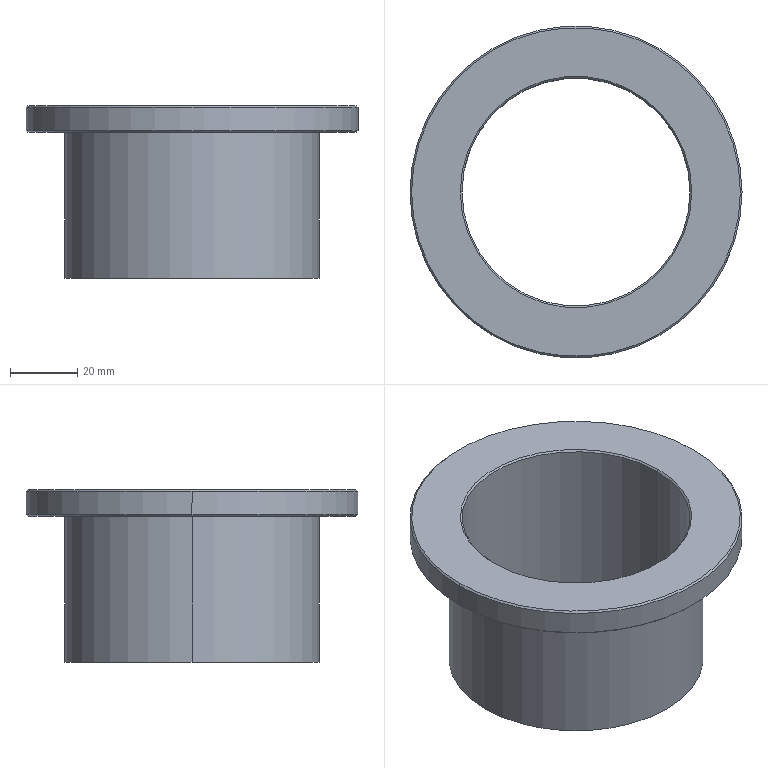Part | STEP file | 7014 Inner Spacer | 1 solid | 15 faces | box 99 x 99 x 51.5 mm | volume 71782 mm3 | cylinder 6 | cone 6 | plane 3 | commonest cylinder face diameters 68 x2 76 x2 99 x2
STEP:
#1=CARTESIAN_POINT('',(34.,0.,51.));
#2=VERTEX_POINT('',#1);
#3=CARTESIAN_POINT('',(-34.,0.,51.));
#4=VERTEX_POINT('',#3);
#5=CARTESIAN_POINT('',(0.,0.,51.));
#6=DIRECTION('',(0.,0.,-1.));
#7=DIRECTION('',(-1.,0.,0.));
#8=AXIS2_PLACEMENT_3D('',#5,#6,#7);
#9=CIRCLE('',#8,34.);
#10=EDGE_CURVE('',#2,#4,#9,.T.);
#11=ORIENTED_EDGE('',*,*,#10,.F.);
#12=CARTESIAN_POINT('',(34.,0.,0.));
#13=VERTEX_POINT('',#12);
#14=CARTESIAN_POINT('',(34.,0.,43.5));
#15=DIRECTION('',(0.,0.,-1.));
#16=VECTOR('',#15,1000.);
#17=LINE('',#14,#16);
#18=EDGE_CURVE('',#2,#13,#17,.T.);
#19=ORIENTED_EDGE('',*,*,#18,.T.);
#20=CARTESIAN_POINT('',(-34.,0.,0.));
#21=VERTEX_POINT('',#20);
#22=CARTESIAN_POINT('',(0.,0.,0.));
#23=DIRECTION('',(0.,0.,1.));
#24=DIRECTION('',(-1.,0.,0.));
#25=AXIS2_PLACEMENT_3D('',#22,#23,#24);
#26=CIRCLE('',#25,34.);
#27=EDGE_CURVE('',#21,#13,#26,.T.);
#28=ORIENTED_EDGE('',*,*,#27,.F.);
#29=CARTESIAN_POINT('',(-34.,0.,43.5));
#30=DIRECTION('',(0.,0.,-1.));
#31=VECTOR('',#30,1000.);
#32=LINE('',#29,#31);
#33=EDGE_CURVE('',#4,#21,#32,.T.);
#34=ORIENTED_EDGE('',*,*,#33,.F.);
#35=EDGE_LOOP('',(#11,#19,#28,#34));
#36=FACE_OUTER_BOUND('',#35,.T.);
#37=CARTESIAN_POINT('',(0.,0.,43.5));
#38=DIRECTION('',(0.,0.,-1.));
#39=DIRECTION('',(-1.,0.,0.));
#40=AXIS2_PLACEMENT_3D('',#37,#38,#39);
#41=CYLINDRICAL_SURFACE('',#40,34.);
#42=ADVANCED_FACE('',(#36),#41,.F.);
#43=ORIENTED_EDGE('',*,*,#10,.T.);
#44=CARTESIAN_POINT('',(-34.5,0.,51.5));
#45=VERTEX_POINT('',#44);
#46=CARTESIAN_POINT('',(-34.5,0.,51.5));
#47=DIRECTION('',(-0.7071,0.,0.7071));
#48=VECTOR('',#47,1000.);
#49=LINE('',#46,#48);
#50=EDGE_CURVE('',#4,#45,#49,.T.);
#51=ORIENTED_EDGE('',*,*,#50,.T.);
#52=CARTESIAN_POINT('',(34.5,0.,51.5));
#53=VERTEX_POINT('',#52);
#54=CARTESIAN_POINT('',(0.,0.,51.5));
#55=DIRECTION('',(0.,0.,-1.));
#56=DIRECTION('',(1.,0.,0.));
#57=AXIS2_PLACEMENT_3D('',#54,#55,#56);
#58=CIRCLE('',#57,34.5);
#59=EDGE_CURVE('',#53,#45,#58,.T.);
#60=ORIENTED_EDGE('',*,*,#59,.F.);
#61=CARTESIAN_POINT('',(34.5,0.,51.5));
#62=DIRECTION('',(0.7071,0.,0.7071));
#63=VECTOR('',#62,1000.);
#64=LINE('',#61,#63);
#65=EDGE_CURVE('',#2,#53,#64,.T.);
#66=ORIENTED_EDGE('',*,*,#65,.F.);
#67=EDGE_LOOP('',(#43,#51,#60,#66));
#68=FACE_OUTER_BOUND('',#67,.T.);
#69=CARTESIAN_POINT('',(0.,0.,51.5));
#70=DIRECTION('',(0.,0.,1.));
#71=DIRECTION('',(1.,0.,0.));
#72=AXIS2_PLACEMENT_3D('',#69,#70,#71);
#73=CONICAL_SURFACE('',#72,34.5,0.7854);
#74=ADVANCED_FACE('',(#68),#73,.F.);
#75=CARTESIAN_POINT('',(-38.,0.,43.5));
#76=VERTEX_POINT('',#75);
#77=CARTESIAN_POINT('',(38.,0.,43.5));
#78=VERTEX_POINT('',#77);
#79=CARTESIAN_POINT('',(0.,0.,43.5));
#80=DIRECTION('',(0.,0.,-1.));
#81=DIRECTION('',(-1.,0.,0.));
#82=AXIS2_PLACEMENT_3D('',#79,#80,#81);
#83=CIRCLE('',#82,38.);
#84=EDGE_CURVE('',#76,#78,#83,.T.);
#85=ORIENTED_EDGE('',*,*,#84,.T.);
#86=CARTESIAN_POINT('',(38.,0.,0.));
#87=VERTEX_POINT('',#86);
#88=CARTESIAN_POINT('',(38.,0.,43.5));
#89=DIRECTION('',(0.,0.,-1.));
#90=VECTOR('',#89,1000.);
#91=LINE('',#88,#90);
#92=EDGE_CURVE('',#78,#87,#91,.T.);
#93=ORIENTED_EDGE('',*,*,#92,.T.);
#94=CARTESIAN_POINT('',(-38.,0.,0.));
#95=VERTEX_POINT('',#94);
#96=CARTESIAN_POINT('',(0.,0.,0.));
#97=DIRECTION('',(0.,0.,1.));
#98=DIRECTION('',(-1.,0.,0.));
#99=AXIS2_PLACEMENT_3D('',#96,#97,#98);
#100=CIRCLE('',#99,38.);
#101=EDGE_CURVE('',#87,#95,#100,.T.);
#102=ORIENTED_EDGE('',*,*,#101,.T.);
#103=CARTESIAN_POINT('',(-38.,0.,43.5));
#104=DIRECTION('',(0.,0.,-1.));
#105=VECTOR('',#104,1000.);
#106=LINE('',#103,#105);
#107=EDGE_CURVE('',#76,#95,#106,.T.);
#108=ORIENTED_EDGE('',*,*,#107,.F.);
#109=EDGE_LOOP('',(#85,#93,#102,#108));
#110=FACE_OUTER_BOUND('',#109,.T.);
#111=CARTESIAN_POINT('',(0.,0.,43.5));
#112=DIRECTION('',(0.,0.,-1.));
#113=DIRECTION('',(-1.,0.,0.));
#114=AXIS2_PLACEMENT_3D('',#111,#112,#113);
#115=CYLINDRICAL_SURFACE('',#114,38.);
#116=ADVANCED_FACE('',(#110),#115,.T.);
#117=CARTESIAN_POINT('',(49.,0.,51.5));
#118=VERTEX_POINT('',#117);
#119=CARTESIAN_POINT('',(-49.,0.,51.5));
#120=VERTEX_POINT('',#119);
#121=CARTESIAN_POINT('',(0.,0.,51.5));
#122=DIRECTION('',(0.,0.,1.));
#123=DIRECTION('',(-1.,0.,0.));
#124=AXIS2_PLACEMENT_3D('',#121,#122,#123);
#125=CIRCLE('',#124,49.);
#126=EDGE_CURVE('',#118,#120,#125,.T.);
#127=ORIENTED_EDGE('',*,*,#126,.F.);
#128=CARTESIAN_POINT('',(49.5,0.,51.));
#129=VERTEX_POINT('',#128);
#130=CARTESIAN_POINT('',(49.5,0.,51.));
#131=DIRECTION('',(0.7071,0.,-0.7071));
#132=VECTOR('',#131,1000.);
#133=LINE('',#130,#132);
#134=EDGE_CURVE('',#118,#129,#133,.T.);
#135=ORIENTED_EDGE('',*,*,#134,.T.);
#136=CARTESIAN_POINT('',(-49.5,0.,51.));
#137=VERTEX_POINT('',#136);
#138=CARTESIAN_POINT('',(0.,0.,51.));
#139=DIRECTION('',(0.,0.,1.));
#140=DIRECTION('',(-1.,0.,0.));
#141=AXIS2_PLACEMENT_3D('',#138,#139,#140);
#142=CIRCLE('',#141,49.5);
#143=EDGE_CURVE('',#129,#137,#142,.T.);
#144=ORIENTED_EDGE('',*,*,#143,.T.);
#145=CARTESIAN_POINT('',(-49.5,0.,51.));
#146=DIRECTION('',(-0.7071,0.,-0.7071));
#147=VECTOR('',#146,1000.);
#148=LINE('',#145,#147);
#149=EDGE_CURVE('',#120,#137,#148,.T.);
#150=ORIENTED_EDGE('',*,*,#149,.F.);
#151=EDGE_LOOP('',(#127,#135,#144,#150));
#152=FACE_OUTER_BOUND('',#151,.T.);
#153=CARTESIAN_POINT('',(0.,0.,51.));
#154=DIRECTION('',(0.,0.,-1.));
#155=DIRECTION('',(-1.,0.,0.));
#156=AXIS2_PLACEMENT_3D('',#153,#154,#155);
#157=CONICAL_SURFACE('',#156,49.5,0.7854);
#158=ADVANCED_FACE('',(#152),#157,.T.);
#159=ORIENTED_EDGE('',*,*,#143,.F.);
#160=CARTESIAN_POINT('',(49.5,0.,44.));
#161=VERTEX_POINT('',#160);
#162=CARTESIAN_POINT('',(49.5,0.,51.5));
#163=DIRECTION('',(0.,0.,-1.));
#164=VECTOR('',#163,1000.);
#165=LINE('',#162,#164);
#166=EDGE_CURVE('',#129,#161,#165,.T.);
#167=ORIENTED_EDGE('',*,*,#166,.T.);
#168=CARTESIAN_POINT('',(-49.5,0.,44.));
#169=VERTEX_POINT('',#168);
#170=CARTESIAN_POINT('',(0.,0.,44.));
#171=DIRECTION('',(0.,0.,1.));
#172=DIRECTION('',(-1.,0.,0.));
#173=AXIS2_PLACEMENT_3D('',#170,#171,#172);
#174=CIRCLE('',#173,49.5);
#175=EDGE_CURVE('',#161,#169,#174,.T.);
#176=ORIENTED_EDGE('',*,*,#175,.T.);
#177=CARTESIAN_POINT('',(-49.5,0.,51.5));
#178=DIRECTION('',(0.,0.,-1.));
#179=VECTOR('',#178,1000.);
#180=LINE('',#177,#179);
#181=EDGE_CURVE('',#137,#169,#180,.T.);
#182=ORIENTED_EDGE('',*,*,#181,.F.);
#183=EDGE_LOOP('',(#159,#167,#176,#182));
#184=FACE_OUTER_BOUND('',#183,.T.);
#185=CARTESIAN_POINT('',(0.,0.,51.5));
#186=DIRECTION('',(0.,0.,-1.));
#187=DIRECTION('',(-1.,0.,0.));
#188=AXIS2_PLACEMENT_3D('',#185,#186,#187);
#189=CYLINDRICAL_SURFACE('',#188,49.5);
#190=ADVANCED_FACE('',(#184),#189,.T.);
#191=CARTESIAN_POINT('',(49.,0.,43.5));
#192=VERTEX_POINT('',#191);
#193=CARTESIAN_POINT('',(-49.,0.,43.5));
#194=VERTEX_POINT('',#193);
#195=CARTESIAN_POINT('',(0.,0.,43.5));
#196=DIRECTION('',(0.,0.,1.));
#197=DIRECTION('',(1.,0.,0.));
#198=AXIS2_PLACEMENT_3D('',#195,#196,#197);
#199=CIRCLE('',#198,49.);
#200=EDGE_CURVE('',#192,#194,#199,.T.);
#201=ORIENTED_EDGE('',*,*,#200,.T.);
#202=CARTESIAN_POINT('',(-49.5,0.,44.));
#203=DIRECTION('',(-0.7071,0.,0.7071));
#204=VECTOR('',#203,1000.);
#205=LINE('',#202,#204);
#206=EDGE_CURVE('',#194,#169,#205,.T.);
#207=ORIENTED_EDGE('',*,*,#206,.T.);
#208=ORIENTED_EDGE('',*,*,#175,.F.);
#209=CARTESIAN_POINT('',(49.5,0.,44.));
#210=DIRECTION('',(0.7071,0.,0.7071));
#211=VECTOR('',#210,1000.);
#212=LINE('',#209,#211);
#213=EDGE_CURVE('',#192,#161,#212,.T.);
#214=ORIENTED_EDGE('',*,*,#213,.F.);
#215=EDGE_LOOP('',(#201,#207,#208,#214));
#216=FACE_OUTER_BOUND('',#215,.T.);
#217=CARTESIAN_POINT('',(0.,0.,44.));
#218=DIRECTION('',(0.,0.,1.));
#219=DIRECTION('',(1.,0.,0.));
#220=AXIS2_PLACEMENT_3D('',#217,#218,#219);
#221=CONICAL_SURFACE('',#220,49.5,0.7854);
#222=ADVANCED_FACE('',(#216),#221,.T.);
#223=ORIENTED_EDGE('',*,*,#18,.F.);
#224=CARTESIAN_POINT('',(0.,0.,51.));
#225=DIRECTION('',(0.,0.,-1.));
#226=DIRECTION('',(-1.,0.,0.));
#227=AXIS2_PLACEMENT_3D('',#224,#225,#226);
#228=CIRCLE('',#227,34.);
#229=EDGE_CURVE('',#4,#2,#228,.T.);
#230=ORIENTED_EDGE('',*,*,#229,.F.);
#231=ORIENTED_EDGE('',*,*,#33,.T.);
#232=CARTESIAN_POINT('',(0.,0.,0.));
#233=DIRECTION('',(0.,0.,1.));
#234=DIRECTION('',(-1.,0.,0.));
#235=AXIS2_PLACEMENT_3D('',#232,#233,#234);
#236=CIRCLE('',#235,34.);
#237=EDGE_CURVE('',#13,#21,#236,.T.);
#238=ORIENTED_EDGE('',*,*,#237,.F.);
#239=EDGE_LOOP('',(#223,#230,#231,#238));
#240=FACE_OUTER_BOUND('',#239,.T.);
#241=CARTESIAN_POINT('',(0.,0.,43.5));
#242=DIRECTION('',(0.,0.,-1.));
#243=DIRECTION('',(-1.,0.,0.));
#244=AXIS2_PLACEMENT_3D('',#241,#242,#243);
#245=CYLINDRICAL_SURFACE('',#244,34.);
#246=ADVANCED_FACE('',(#240),#245,.F.);
#247=ORIENTED_EDGE('',*,*,#50,.F.);
#248=ORIENTED_EDGE('',*,*,#229,.T.);
#249=ORIENTED_EDGE('',*,*,#65,.T.);
#250=CARTESIAN_POINT('',(0.,0.,51.5));
#251=DIRECTION('',(0.,0.,-1.));
#252=DIRECTION('',(1.,0.,0.));
#253=AXIS2_PLACEMENT_3D('',#250,#251,#252);
#254=CIRCLE('',#253,34.5);
#255=EDGE_CURVE('',#45,#53,#254,.T.);
#256=ORIENTED_EDGE('',*,*,#255,.F.);
#257=EDGE_LOOP('',(#247,#248,#249,#256));
#258=FACE_OUTER_BOUND('',#257,.T.);
#259=CARTESIAN_POINT('',(0.,0.,51.5));
#260=DIRECTION('',(0.,0.,1.));
#261=DIRECTION('',(1.,0.,0.));
#262=AXIS2_PLACEMENT_3D('',#259,#260,#261);
#263=CONICAL_SURFACE('',#262,34.5,0.7854);
#264=ADVANCED_FACE('',(#258),#263,.F.);
#265=ORIENTED_EDGE('',*,*,#27,.T.);
#266=ORIENTED_EDGE('',*,*,#237,.T.);
#267=EDGE_LOOP('',(#265,#266));
#268=FACE_BOUND('',#267,.T.);
#269=CARTESIAN_POINT('',(0.,0.,0.));
#270=DIRECTION('',(0.,0.,1.));
#271=DIRECTION('',(-1.,0.,0.));
#272=AXIS2_PLACEMENT_3D('',#269,#270,#271);
#273=CIRCLE('',#272,38.);
#274=EDGE_CURVE('',#95,#87,#273,.T.);
#275=ORIENTED_EDGE('',*,*,#274,.F.);
#276=ORIENTED_EDGE('',*,*,#101,.F.);
#277=EDGE_LOOP('',(#275,#276));
#278=FACE_OUTER_BOUND('',#277,.T.);
#279=CARTESIAN_POINT('',(0.,0.,0.));
#280=DIRECTION('',(0.,0.,1.));
#281=DIRECTION('',(1.,0.,0.));
#282=AXIS2_PLACEMENT_3D('',#279,#280,#281);
#283=PLANE('',#282);
#284=ADVANCED_FACE('',(#268,#278),#283,.F.);
#285=ORIENTED_EDGE('',*,*,#59,.T.);
#286=ORIENTED_EDGE('',*,*,#255,.T.);
#287=EDGE_LOOP('',(#285,#286));
#288=FACE_BOUND('',#287,.T.);
#289=CARTESIAN_POINT('',(0.,0.,51.5));
#290=DIRECTION('',(0.,0.,1.));
#291=DIRECTION('',(-1.,0.,0.));
#292=AXIS2_PLACEMENT_3D('',#289,#290,#291);
#293=CIRCLE('',#292,49.);
#294=EDGE_CURVE('',#120,#118,#293,.T.);
#295=ORIENTED_EDGE('',*,*,#294,.T.);
#296=ORIENTED_EDGE('',*,*,#126,.T.);
#297=EDGE_LOOP('',(#295,#296));
#298=FACE_OUTER_BOUND('',#297,.T.);
#299=CARTESIAN_POINT('',(0.,0.,51.5));
#300=DIRECTION('',(0.,0.,1.));
#301=DIRECTION('',(1.,0.,0.));
#302=AXIS2_PLACEMENT_3D('',#299,#300,#301);
#303=PLANE('',#302);
#304=ADVANCED_FACE('',(#288,#298),#303,.T.);
#305=ORIENTED_EDGE('',*,*,#92,.F.);
#306=CARTESIAN_POINT('',(0.,0.,43.5));
#307=DIRECTION('',(0.,0.,-1.));
#308=DIRECTION('',(-1.,0.,0.));
#309=AXIS2_PLACEMENT_3D('',#306,#307,#308);
#310=CIRCLE('',#309,38.);
#311=EDGE_CURVE('',#78,#76,#310,.T.);
#312=ORIENTED_EDGE('',*,*,#311,.T.);
#313=ORIENTED_EDGE('',*,*,#107,.T.);
#314=ORIENTED_EDGE('',*,*,#274,.T.);
#315=EDGE_LOOP('',(#305,#312,#313,#314));
#316=FACE_OUTER_BOUND('',#315,.T.);
#317=CARTESIAN_POINT('',(0.,0.,43.5));
#318=DIRECTION('',(0.,0.,-1.));
#319=DIRECTION('',(-1.,0.,0.));
#320=AXIS2_PLACEMENT_3D('',#317,#318,#319);
#321=CYLINDRICAL_SURFACE('',#320,38.);
#322=ADVANCED_FACE('',(#316),#321,.T.);
#323=ORIENTED_EDGE('',*,*,#134,.F.);
#324=ORIENTED_EDGE('',*,*,#294,.F.);
#325=ORIENTED_EDGE('',*,*,#149,.T.);
#326=CARTESIAN_POINT('',(0.,0.,51.));
#327=DIRECTION('',(0.,0.,1.));
#328=DIRECTION('',(-1.,0.,0.));
#329=AXIS2_PLACEMENT_3D('',#326,#327,#328);
#330=CIRCLE('',#329,49.5);
#331=EDGE_CURVE('',#137,#129,#330,.T.);
#332=ORIENTED_EDGE('',*,*,#331,.T.);
#333=EDGE_LOOP('',(#323,#324,#325,#332));
#334=FACE_OUTER_BOUND('',#333,.T.);
#335=CARTESIAN_POINT('',(0.,0.,51.));
#336=DIRECTION('',(0.,0.,-1.));
#337=DIRECTION('',(-1.,0.,0.));
#338=AXIS2_PLACEMENT_3D('',#335,#336,#337);
#339=CONICAL_SURFACE('',#338,49.5,0.7854);
#340=ADVANCED_FACE('',(#334),#339,.T.);
#341=ORIENTED_EDGE('',*,*,#84,.F.);
#342=ORIENTED_EDGE('',*,*,#311,.F.);
#343=EDGE_LOOP('',(#341,#342));
#344=FACE_BOUND('',#343,.T.);
#345=ORIENTED_EDGE('',*,*,#200,.F.);
#346=CARTESIAN_POINT('',(0.,0.,43.5));
#347=DIRECTION('',(0.,0.,1.));
#348=DIRECTION('',(1.,0.,0.));
#349=AXIS2_PLACEMENT_3D('',#346,#347,#348);
#350=CIRCLE('',#349,49.);
#351=EDGE_CURVE('',#194,#192,#350,.T.);
#352=ORIENTED_EDGE('',*,*,#351,.F.);
#353=EDGE_LOOP('',(#345,#352));
#354=FACE_OUTER_BOUND('',#353,.T.);
#355=CARTESIAN_POINT('',(0.,0.,43.5));
#356=DIRECTION('',(0.,0.,1.));
#357=DIRECTION('',(1.,0.,0.));
#358=AXIS2_PLACEMENT_3D('',#355,#356,#357);
#359=PLANE('',#358);
#360=ADVANCED_FACE('',(#344,#354),#359,.F.);
#361=ORIENTED_EDGE('',*,*,#166,.F.);
#362=ORIENTED_EDGE('',*,*,#331,.F.);
#363=ORIENTED_EDGE('',*,*,#181,.T.);
#364=CARTESIAN_POINT('',(0.,0.,44.));
#365=DIRECTION('',(0.,0.,1.));
#366=DIRECTION('',(-1.,0.,0.));
#367=AXIS2_PLACEMENT_3D('',#364,#365,#366);
#368=CIRCLE('',#367,49.5);
#369=EDGE_CURVE('',#169,#161,#368,.T.);
#370=ORIENTED_EDGE('',*,*,#369,.T.);
#371=EDGE_LOOP('',(#361,#362,#363,#370));
#372=FACE_OUTER_BOUND('',#371,.T.);
#373=CARTESIAN_POINT('',(0.,0.,51.5));
#374=DIRECTION('',(0.,0.,-1.));
#375=DIRECTION('',(-1.,0.,0.));
#376=AXIS2_PLACEMENT_3D('',#373,#374,#375);
#377=CYLINDRICAL_SURFACE('',#376,49.5);
#378=ADVANCED_FACE('',(#372),#377,.T.);
#379=ORIENTED_EDGE('',*,*,#206,.F.);
#380=ORIENTED_EDGE('',*,*,#351,.T.);
#381=ORIENTED_EDGE('',*,*,#213,.T.);
#382=ORIENTED_EDGE('',*,*,#369,.F.);
#383=EDGE_LOOP('',(#379,#380,#381,#382));
#384=FACE_OUTER_BOUND('',#383,.T.);
#385=CARTESIAN_POINT('',(0.,0.,44.));
#386=DIRECTION('',(0.,0.,1.));
#387=DIRECTION('',(1.,0.,0.));
#388=AXIS2_PLACEMENT_3D('',#385,#386,#387);
#389=CONICAL_SURFACE('',#388,49.5,0.7854);
#390=ADVANCED_FACE('',(#384),#389,.T.);
#391=CLOSED_SHELL('',(#42,#74,#116,#158,#190,#222,#246,#264,#284,#304,#322,#340,#360,#378,#390));
#392=MANIFOLD_SOLID_BREP('',#391);
#393=CARTESIAN_POINT('',(0.,0.,0.));
#394=DIRECTION('',(0.,0.,1.));
#395=DIRECTION('',(1.,0.,0.));
#396=AXIS2_PLACEMENT_3D('',#393,#394,#395);
#397=(LENGTH_UNIT()NAMED_UNIT(*)SI_UNIT(.MILLI.,.METRE.));
#398=UNCERTAINTY_MEASURE_WITH_UNIT(LENGTH_MEASURE(0.00001),#397,'','');
#399=(NAMED_UNIT(*)PLANE_ANGLE_UNIT()SI_UNIT($,.RADIAN.));
#400=(NAMED_UNIT(*)SI_UNIT($,.STERADIAN.)SOLID_ANGLE_UNIT());
#401=(GEOMETRIC_REPRESENTATION_CONTEXT(3)GLOBAL_UNCERTAINTY_ASSIGNED_CONTEXT((#398))GLOBAL_UNIT_ASSIGNED_CONTEXT((#397,#399,#400))REPRESENTATION_CONTEXT('',''));
#402=ADVANCED_BREP_SHAPE_REPRESENTATION('',(#392,#396),#401);